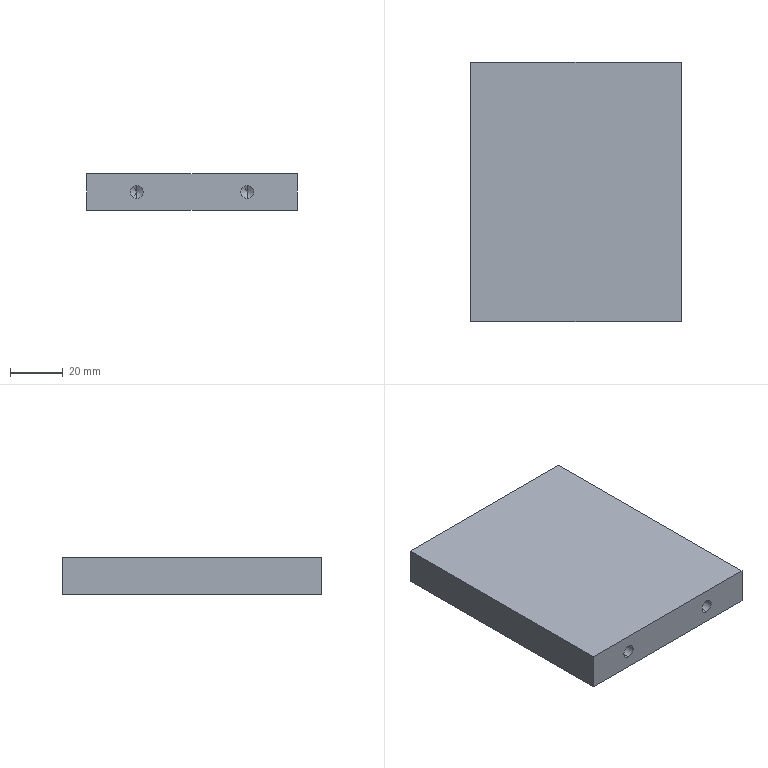Part | SolidWorks | features HoleWzd 2, Extrusion 1 | 1 solid | 22 faces | box 80 x 98.4 x 14 mm | volume 108833 mm3 | cylinder 8 | cone 8 | plane 6 | commonest cylinder face diameters 5 x8
STEP:
#1=CARTESIAN_POINT('',(-17.5,32.2,4.5));
#2=VERTEX_POINT('',#1);
#3=CARTESIAN_POINT('',(-17.5,32.2,9.5));
#4=VERTEX_POINT('',#3);
#5=CARTESIAN_POINT('',(-17.5,32.2,7.));
#6=DIRECTION('',(0.,1.,0.));
#7=DIRECTION('',(0.,0.,1.));
#8=AXIS2_PLACEMENT_3D('',#5,#6,#7);
#9=CIRCLE('',#8,2.5);
#10=EDGE_CURVE('',#2,#4,#9,.T.);
#11=ORIENTED_EDGE('',*,*,#10,.F.);
#12=CARTESIAN_POINT('',(-17.5,49.2,4.5));
#13=VERTEX_POINT('',#12);
#14=CARTESIAN_POINT('',(-17.5,49.2,4.5));
#15=DIRECTION('',(0.,1.,0.));
#16=VECTOR('',#15,1000.);
#17=LINE('',#14,#16);
#18=EDGE_CURVE('',#2,#13,#17,.T.);
#19=ORIENTED_EDGE('',*,*,#18,.T.);
#20=CARTESIAN_POINT('',(-17.5,49.2,9.5));
#21=VERTEX_POINT('',#20);
#22=CARTESIAN_POINT('',(-17.5,49.2,7.));
#23=DIRECTION('',(0.,1.,0.));
#24=DIRECTION('',(0.,0.,1.));
#25=AXIS2_PLACEMENT_3D('',#22,#23,#24);
#26=CIRCLE('',#25,2.5);
#27=EDGE_CURVE('',#13,#21,#26,.T.);
#28=ORIENTED_EDGE('',*,*,#27,.T.);
#29=CARTESIAN_POINT('',(-17.5,49.2,9.5));
#30=DIRECTION('',(0.,1.,0.));
#31=VECTOR('',#30,1000.);
#32=LINE('',#29,#31);
#33=EDGE_CURVE('',#4,#21,#32,.T.);
#34=ORIENTED_EDGE('',*,*,#33,.F.);
#35=EDGE_LOOP('',(#11,#19,#28,#34));
#36=FACE_OUTER_BOUND('',#35,.T.);
#37=CARTESIAN_POINT('',(-17.5,49.2,7.));
#38=DIRECTION('',(0.,1.,0.));
#39=DIRECTION('',(0.,0.,1.));
#40=AXIS2_PLACEMENT_3D('',#37,#38,#39);
#41=CYLINDRICAL_SURFACE('',#40,2.5);
#42=ADVANCED_FACE('',(#36),#41,.F.);
#43=CARTESIAN_POINT('',(-17.5,30.698,7.));
#44=VERTEX_POINT('',#43);
#45=CARTESIAN_POINT('',(-17.5,32.2,9.5));
#46=DIRECTION('',(0.,0.515,0.8572));
#47=VECTOR('',#46,1000.);
#48=LINE('',#45,#47);
#49=EDGE_CURVE('',#44,#4,#48,.T.);
#50=ORIENTED_EDGE('',*,*,#49,.F.);
#51=CARTESIAN_POINT('',(-17.5,32.2,4.5));
#52=DIRECTION('',(0.,0.515,-0.8572));
#53=VECTOR('',#52,1000.);
#54=LINE('',#51,#53);
#55=EDGE_CURVE('',#44,#2,#54,.T.);
#56=ORIENTED_EDGE('',*,*,#55,.T.);
#57=ORIENTED_EDGE('',*,*,#10,.T.);
#58=EDGE_LOOP('',(#50,#56,#57));
#59=FACE_OUTER_BOUND('',#58,.T.);
#60=CARTESIAN_POINT('',(-17.5,32.2,7.));
#61=DIRECTION('',(0.,1.,0.));
#62=DIRECTION('',(0.,0.,1.));
#63=AXIS2_PLACEMENT_3D('',#60,#61,#62);
#64=CONICAL_SURFACE('',#63,2.5,1.03);
#65=ADVANCED_FACE('',(#59),#64,.F.);
#66=CARTESIAN_POINT('',(17.5,32.2,4.5));
#67=VERTEX_POINT('',#66);
#68=CARTESIAN_POINT('',(17.5,32.2,9.5));
#69=VERTEX_POINT('',#68);
#70=CARTESIAN_POINT('',(17.5,32.2,7.));
#71=DIRECTION('',(0.,1.,0.));
#72=DIRECTION('',(0.,0.,1.));
#73=AXIS2_PLACEMENT_3D('',#70,#71,#72);
#74=CIRCLE('',#73,2.5);
#75=EDGE_CURVE('',#67,#69,#74,.T.);
#76=ORIENTED_EDGE('',*,*,#75,.F.);
#77=CARTESIAN_POINT('',(17.5,49.2,4.5));
#78=VERTEX_POINT('',#77);
#79=CARTESIAN_POINT('',(17.5,49.2,4.5));
#80=DIRECTION('',(0.,1.,0.));
#81=VECTOR('',#80,1000.);
#82=LINE('',#79,#81);
#83=EDGE_CURVE('',#67,#78,#82,.T.);
#84=ORIENTED_EDGE('',*,*,#83,.T.);
#85=CARTESIAN_POINT('',(17.5,49.2,9.5));
#86=VERTEX_POINT('',#85);
#87=CARTESIAN_POINT('',(17.5,49.2,7.));
#88=DIRECTION('',(0.,1.,0.));
#89=DIRECTION('',(0.,0.,1.));
#90=AXIS2_PLACEMENT_3D('',#87,#88,#89);
#91=CIRCLE('',#90,2.5);
#92=EDGE_CURVE('',#78,#86,#91,.T.);
#93=ORIENTED_EDGE('',*,*,#92,.T.);
#94=CARTESIAN_POINT('',(17.5,49.2,9.5));
#95=DIRECTION('',(0.,1.,0.));
#96=VECTOR('',#95,1000.);
#97=LINE('',#94,#96);
#98=EDGE_CURVE('',#69,#86,#97,.T.);
#99=ORIENTED_EDGE('',*,*,#98,.F.);
#100=EDGE_LOOP('',(#76,#84,#93,#99));
#101=FACE_OUTER_BOUND('',#100,.T.);
#102=CARTESIAN_POINT('',(17.5,49.2,7.));
#103=DIRECTION('',(0.,1.,0.));
#104=DIRECTION('',(0.,0.,1.));
#105=AXIS2_PLACEMENT_3D('',#102,#103,#104);
#106=CYLINDRICAL_SURFACE('',#105,2.5);
#107=ADVANCED_FACE('',(#101),#106,.F.);
#108=CARTESIAN_POINT('',(17.5,30.698,7.));
#109=VERTEX_POINT('',#108);
#110=CARTESIAN_POINT('',(17.5,32.2,9.5));
#111=DIRECTION('',(0.,0.515,0.8572));
#112=VECTOR('',#111,1000.);
#113=LINE('',#110,#112);
#114=EDGE_CURVE('',#109,#69,#113,.T.);
#115=ORIENTED_EDGE('',*,*,#114,.F.);
#116=CARTESIAN_POINT('',(17.5,32.2,4.5));
#117=DIRECTION('',(0.,0.515,-0.8572));
#118=VECTOR('',#117,1000.);
#119=LINE('',#116,#118);
#120=EDGE_CURVE('',#109,#67,#119,.T.);
#121=ORIENTED_EDGE('',*,*,#120,.T.);
#122=ORIENTED_EDGE('',*,*,#75,.T.);
#123=EDGE_LOOP('',(#115,#121,#122));
#124=FACE_OUTER_BOUND('',#123,.T.);
#125=CARTESIAN_POINT('',(17.5,32.2,7.));
#126=DIRECTION('',(0.,1.,0.));
#127=DIRECTION('',(0.,0.,1.));
#128=AXIS2_PLACEMENT_3D('',#125,#126,#127);
#129=CONICAL_SURFACE('',#128,2.5,1.03);
#130=ADVANCED_FACE('',(#124),#129,.F.);
#131=CARTESIAN_POINT('',(21.,-32.2,9.5));
#132=VERTEX_POINT('',#131);
#133=CARTESIAN_POINT('',(21.,-32.2,4.5));
#134=VERTEX_POINT('',#133);
#135=CARTESIAN_POINT('',(21.,-32.2,7.));
#136=DIRECTION('',(0.,-1.,0.));
#137=DIRECTION('',(0.,0.,-1.));
#138=AXIS2_PLACEMENT_3D('',#135,#136,#137);
#139=CIRCLE('',#138,2.5);
#140=EDGE_CURVE('',#132,#134,#139,.T.);
#141=ORIENTED_EDGE('',*,*,#140,.F.);
#142=CARTESIAN_POINT('',(21.,-49.2,9.5));
#143=VERTEX_POINT('',#142);
#144=CARTESIAN_POINT('',(21.,-49.2,9.5));
#145=DIRECTION('',(0.,-1.,0.));
#146=VECTOR('',#145,1000.);
#147=LINE('',#144,#146);
#148=EDGE_CURVE('',#132,#143,#147,.T.);
#149=ORIENTED_EDGE('',*,*,#148,.T.);
#150=CARTESIAN_POINT('',(21.,-49.2,4.5));
#151=VERTEX_POINT('',#150);
#152=CARTESIAN_POINT('',(21.,-49.2,7.));
#153=DIRECTION('',(0.,-1.,0.));
#154=DIRECTION('',(0.,0.,-1.));
#155=AXIS2_PLACEMENT_3D('',#152,#153,#154);
#156=CIRCLE('',#155,2.5);
#157=EDGE_CURVE('',#143,#151,#156,.T.);
#158=ORIENTED_EDGE('',*,*,#157,.T.);
#159=CARTESIAN_POINT('',(21.,-49.2,4.5));
#160=DIRECTION('',(0.,-1.,0.));
#161=VECTOR('',#160,1000.);
#162=LINE('',#159,#161);
#163=EDGE_CURVE('',#134,#151,#162,.T.);
#164=ORIENTED_EDGE('',*,*,#163,.F.);
#165=EDGE_LOOP('',(#141,#149,#158,#164));
#166=FACE_OUTER_BOUND('',#165,.T.);
#167=CARTESIAN_POINT('',(21.,-49.2,7.));
#168=DIRECTION('',(0.,-1.,0.));
#169=DIRECTION('',(0.,0.,-1.));
#170=AXIS2_PLACEMENT_3D('',#167,#168,#169);
#171=CYLINDRICAL_SURFACE('',#170,2.5);
#172=ADVANCED_FACE('',(#166),#171,.F.);
#173=CARTESIAN_POINT('',(21.,-30.698,7.));
#174=VERTEX_POINT('',#173);
#175=CARTESIAN_POINT('',(21.,-32.2,4.5));
#176=DIRECTION('',(0.,-0.515,-0.8572));
#177=VECTOR('',#176,1000.);
#178=LINE('',#175,#177);
#179=EDGE_CURVE('',#174,#134,#178,.T.);
#180=ORIENTED_EDGE('',*,*,#179,.F.);
#181=CARTESIAN_POINT('',(21.,-32.2,9.5));
#182=DIRECTION('',(0.,-0.515,0.8572));
#183=VECTOR('',#182,1000.);
#184=LINE('',#181,#183);
#185=EDGE_CURVE('',#174,#132,#184,.T.);
#186=ORIENTED_EDGE('',*,*,#185,.T.);
#187=ORIENTED_EDGE('',*,*,#140,.T.);
#188=EDGE_LOOP('',(#180,#186,#187));
#189=FACE_OUTER_BOUND('',#188,.T.);
#190=CARTESIAN_POINT('',(21.,-32.2,7.));
#191=DIRECTION('',(0.,-1.,0.));
#192=DIRECTION('',(0.,0.,-1.));
#193=AXIS2_PLACEMENT_3D('',#190,#191,#192);
#194=CONICAL_SURFACE('',#193,2.5,1.03);
#195=ADVANCED_FACE('',(#189),#194,.F.);
#196=CARTESIAN_POINT('',(-21.,-32.2,9.5));
#197=VERTEX_POINT('',#196);
#198=CARTESIAN_POINT('',(-21.,-32.2,4.5));
#199=VERTEX_POINT('',#198);
#200=CARTESIAN_POINT('',(-21.,-32.2,7.));
#201=DIRECTION('',(0.,-1.,0.));
#202=DIRECTION('',(0.,0.,-1.));
#203=AXIS2_PLACEMENT_3D('',#200,#201,#202);
#204=CIRCLE('',#203,2.5);
#205=EDGE_CURVE('',#197,#199,#204,.T.);
#206=ORIENTED_EDGE('',*,*,#205,.F.);
#207=CARTESIAN_POINT('',(-21.,-49.2,9.5));
#208=VERTEX_POINT('',#207);
#209=CARTESIAN_POINT('',(-21.,-49.2,9.5));
#210=DIRECTION('',(0.,-1.,0.));
#211=VECTOR('',#210,1000.);
#212=LINE('',#209,#211);
#213=EDGE_CURVE('',#197,#208,#212,.T.);
#214=ORIENTED_EDGE('',*,*,#213,.T.);
#215=CARTESIAN_POINT('',(-21.,-49.2,4.5));
#216=VERTEX_POINT('',#215);
#217=CARTESIAN_POINT('',(-21.,-49.2,7.));
#218=DIRECTION('',(0.,-1.,0.));
#219=DIRECTION('',(0.,0.,-1.));
#220=AXIS2_PLACEMENT_3D('',#217,#218,#219);
#221=CIRCLE('',#220,2.5);
#222=EDGE_CURVE('',#208,#216,#221,.T.);
#223=ORIENTED_EDGE('',*,*,#222,.T.);
#224=CARTESIAN_POINT('',(-21.,-49.2,4.5));
#225=DIRECTION('',(0.,-1.,0.));
#226=VECTOR('',#225,1000.);
#227=LINE('',#224,#226);
#228=EDGE_CURVE('',#199,#216,#227,.T.);
#229=ORIENTED_EDGE('',*,*,#228,.F.);
#230=EDGE_LOOP('',(#206,#214,#223,#229));
#231=FACE_OUTER_BOUND('',#230,.T.);
#232=CARTESIAN_POINT('',(-21.,-49.2,7.));
#233=DIRECTION('',(0.,-1.,0.));
#234=DIRECTION('',(0.,0.,-1.));
#235=AXIS2_PLACEMENT_3D('',#232,#233,#234);
#236=CYLINDRICAL_SURFACE('',#235,2.5);
#237=ADVANCED_FACE('',(#231),#236,.F.);
#238=CARTESIAN_POINT('',(-21.,-30.698,7.));
#239=VERTEX_POINT('',#238);
#240=CARTESIAN_POINT('',(-21.,-32.2,4.5));
#241=DIRECTION('',(0.,-0.515,-0.8572));
#242=VECTOR('',#241,1000.);
#243=LINE('',#240,#242);
#244=EDGE_CURVE('',#239,#199,#243,.T.);
#245=ORIENTED_EDGE('',*,*,#244,.F.);
#246=CARTESIAN_POINT('',(-21.,-32.2,9.5));
#247=DIRECTION('',(0.,-0.515,0.8572));
#248=VECTOR('',#247,1000.);
#249=LINE('',#246,#248);
#250=EDGE_CURVE('',#239,#197,#249,.T.);
#251=ORIENTED_EDGE('',*,*,#250,.T.);
#252=ORIENTED_EDGE('',*,*,#205,.T.);
#253=EDGE_LOOP('',(#245,#251,#252));
#254=FACE_OUTER_BOUND('',#253,.T.);
#255=CARTESIAN_POINT('',(-21.,-32.2,7.));
#256=DIRECTION('',(0.,-1.,0.));
#257=DIRECTION('',(0.,0.,-1.));
#258=AXIS2_PLACEMENT_3D('',#255,#256,#257);
#259=CONICAL_SURFACE('',#258,2.5,1.03);
#260=ADVANCED_FACE('',(#254),#259,.F.);
#261=CARTESIAN_POINT('',(40.,-49.2,0.));
#262=VERTEX_POINT('',#261);
#263=CARTESIAN_POINT('',(40.,49.2,0.));
#264=VERTEX_POINT('',#263);
#265=CARTESIAN_POINT('',(40.,49.2,0.));
#266=DIRECTION('',(0.,1.,0.));
#267=VECTOR('',#266,1000.);
#268=LINE('',#265,#267);
#269=EDGE_CURVE('',#262,#264,#268,.T.);
#270=ORIENTED_EDGE('',*,*,#269,.T.);
#271=CARTESIAN_POINT('',(40.,49.2,14.));
#272=VERTEX_POINT('',#271);
#273=CARTESIAN_POINT('',(40.,49.2,14.));
#274=DIRECTION('',(0.,0.,-1.));
#275=VECTOR('',#274,1000.);
#276=LINE('',#273,#275);
#277=EDGE_CURVE('',#272,#264,#276,.T.);
#278=ORIENTED_EDGE('',*,*,#277,.F.);
#279=CARTESIAN_POINT('',(40.,-49.2,14.));
#280=VERTEX_POINT('',#279);
#281=CARTESIAN_POINT('',(40.,49.2,14.));
#282=DIRECTION('',(0.,1.,0.));
#283=VECTOR('',#282,1000.);
#284=LINE('',#281,#283);
#285=EDGE_CURVE('',#280,#272,#284,.T.);
#286=ORIENTED_EDGE('',*,*,#285,.F.);
#287=CARTESIAN_POINT('',(40.,-49.2,14.));
#288=DIRECTION('',(0.,0.,-1.));
#289=VECTOR('',#288,1000.);
#290=LINE('',#287,#289);
#291=EDGE_CURVE('',#280,#262,#290,.T.);
#292=ORIENTED_EDGE('',*,*,#291,.T.);
#293=EDGE_LOOP('',(#270,#278,#286,#292));
#294=FACE_OUTER_BOUND('',#293,.T.);
#295=CARTESIAN_POINT('',(40.,49.2,14.));
#296=DIRECTION('',(-1.,0.,0.));
#297=DIRECTION('',(0.,-1.,0.));
#298=AXIS2_PLACEMENT_3D('',#295,#296,#297);
#299=PLANE('',#298);
#300=ADVANCED_FACE('',(#294),#299,.F.);
#301=CARTESIAN_POINT('',(-17.5,49.2,7.));
#302=DIRECTION('',(0.,1.,0.));
#303=DIRECTION('',(0.,0.,1.));
#304=AXIS2_PLACEMENT_3D('',#301,#302,#303);
#305=CIRCLE('',#304,2.5);
#306=EDGE_CURVE('',#21,#13,#305,.T.);
#307=ORIENTED_EDGE('',*,*,#306,.F.);
#308=ORIENTED_EDGE('',*,*,#27,.F.);
#309=EDGE_LOOP('',(#307,#308));
#310=FACE_BOUND('',#309,.T.);
#311=CARTESIAN_POINT('',(17.5,49.2,7.));
#312=DIRECTION('',(0.,1.,0.));
#313=DIRECTION('',(0.,0.,1.));
#314=AXIS2_PLACEMENT_3D('',#311,#312,#313);
#315=CIRCLE('',#314,2.5);
#316=EDGE_CURVE('',#86,#78,#315,.T.);
#317=ORIENTED_EDGE('',*,*,#316,.F.);
#318=ORIENTED_EDGE('',*,*,#92,.F.);
#319=EDGE_LOOP('',(#317,#318));
#320=FACE_BOUND('',#319,.T.);
#321=CARTESIAN_POINT('',(-40.,49.2,0.));
#322=VERTEX_POINT('',#321);
#323=CARTESIAN_POINT('',(-40.,49.2,0.));
#324=DIRECTION('',(-1.,0.,0.));
#325=VECTOR('',#324,1000.);
#326=LINE('',#323,#325);
#327=EDGE_CURVE('',#264,#322,#326,.T.);
#328=ORIENTED_EDGE('',*,*,#327,.T.);
#329=CARTESIAN_POINT('',(-40.,49.2,14.));
#330=VERTEX_POINT('',#329);
#331=CARTESIAN_POINT('',(-40.,49.2,14.));
#332=DIRECTION('',(0.,0.,-1.));
#333=VECTOR('',#332,1000.);
#334=LINE('',#331,#333);
#335=EDGE_CURVE('',#330,#322,#334,.T.);
#336=ORIENTED_EDGE('',*,*,#335,.F.);
#337=CARTESIAN_POINT('',(-40.,49.2,14.));
#338=DIRECTION('',(-1.,0.,0.));
#339=VECTOR('',#338,1000.);
#340=LINE('',#337,#339);
#341=EDGE_CURVE('',#272,#330,#340,.T.);
#342=ORIENTED_EDGE('',*,*,#341,.F.);
#343=ORIENTED_EDGE('',*,*,#277,.T.);
#344=EDGE_LOOP('',(#328,#336,#342,#343));
#345=FACE_OUTER_BOUND('',#344,.T.);
#346=CARTESIAN_POINT('',(-40.,49.2,14.));
#347=DIRECTION('',(0.,-1.,0.));
#348=DIRECTION('',(0.,0.,-1.));
#349=AXIS2_PLACEMENT_3D('',#346,#347,#348);
#350=PLANE('',#349);
#351=ADVANCED_FACE('',(#310,#320,#345),#350,.F.);
#352=CARTESIAN_POINT('',(-40.,-49.2,0.));
#353=VERTEX_POINT('',#352);
#354=CARTESIAN_POINT('',(-40.,49.2,0.));
#355=DIRECTION('',(0.,-1.,0.));
#356=VECTOR('',#355,1000.);
#357=LINE('',#354,#356);
#358=EDGE_CURVE('',#322,#353,#357,.T.);
#359=ORIENTED_EDGE('',*,*,#358,.T.);
#360=CARTESIAN_POINT('',(-40.,-49.2,14.));
#361=VERTEX_POINT('',#360);
#362=CARTESIAN_POINT('',(-40.,-49.2,14.));
#363=DIRECTION('',(0.,0.,-1.));
#364=VECTOR('',#363,1000.);
#365=LINE('',#362,#364);
#366=EDGE_CURVE('',#361,#353,#365,.T.);
#367=ORIENTED_EDGE('',*,*,#366,.F.);
#368=CARTESIAN_POINT('',(-40.,49.2,14.));
#369=DIRECTION('',(0.,-1.,0.));
#370=VECTOR('',#369,1000.);
#371=LINE('',#368,#370);
#372=EDGE_CURVE('',#330,#361,#371,.T.);
#373=ORIENTED_EDGE('',*,*,#372,.F.);
#374=ORIENTED_EDGE('',*,*,#335,.T.);
#375=EDGE_LOOP('',(#359,#367,#373,#374));
#376=FACE_OUTER_BOUND('',#375,.T.);
#377=CARTESIAN_POINT('',(-40.,49.2,14.));
#378=DIRECTION('',(1.,0.,0.));
#379=DIRECTION('',(0.,1.,0.));
#380=AXIS2_PLACEMENT_3D('',#377,#378,#379);
#381=PLANE('',#380);
#382=ADVANCED_FACE('',(#376),#381,.F.);
#383=CARTESIAN_POINT('',(21.,-49.2,7.));
#384=DIRECTION('',(0.,-1.,0.));
#385=DIRECTION('',(0.,0.,-1.));
#386=AXIS2_PLACEMENT_3D('',#383,#384,#385);
#387=CIRCLE('',#386,2.5);
#388=EDGE_CURVE('',#151,#143,#387,.T.);
#389=ORIENTED_EDGE('',*,*,#388,.F.);
#390=ORIENTED_EDGE('',*,*,#157,.F.);
#391=EDGE_LOOP('',(#389,#390));
#392=FACE_BOUND('',#391,.T.);
#393=CARTESIAN_POINT('',(-21.,-49.2,7.));
#394=DIRECTION('',(0.,-1.,0.));
#395=DIRECTION('',(0.,0.,-1.));
#396=AXIS2_PLACEMENT_3D('',#393,#394,#395);
#397=CIRCLE('',#396,2.5);
#398=EDGE_CURVE('',#216,#208,#397,.T.);
#399=ORIENTED_EDGE('',*,*,#398,.F.);
#400=ORIENTED_EDGE('',*,*,#222,.F.);
#401=EDGE_LOOP('',(#399,#400));
#402=FACE_BOUND('',#401,.T.);
#403=CARTESIAN_POINT('',(-40.,-49.2,0.));
#404=DIRECTION('',(1.,0.,0.));
#405=VECTOR('',#404,1000.);
#406=LINE('',#403,#405);
#407=EDGE_CURVE('',#353,#262,#406,.T.);
#408=ORIENTED_EDGE('',*,*,#407,.T.);
#409=ORIENTED_EDGE('',*,*,#291,.F.);
#410=CARTESIAN_POINT('',(-40.,-49.2,14.));
#411=DIRECTION('',(1.,0.,0.));
#412=VECTOR('',#411,1000.);
#413=LINE('',#410,#412);
#414=EDGE_CURVE('',#361,#280,#413,.T.);
#415=ORIENTED_EDGE('',*,*,#414,.F.);
#416=ORIENTED_EDGE('',*,*,#366,.T.);
#417=EDGE_LOOP('',(#408,#409,#415,#416));
#418=FACE_OUTER_BOUND('',#417,.T.);
#419=CARTESIAN_POINT('',(-40.,-49.2,14.));
#420=DIRECTION('',(0.,1.,0.));
#421=DIRECTION('',(0.,0.,1.));
#422=AXIS2_PLACEMENT_3D('',#419,#420,#421);
#423=PLANE('',#422);
#424=ADVANCED_FACE('',(#392,#402,#418),#423,.F.);
#425=ORIENTED_EDGE('',*,*,#285,.T.);
#426=ORIENTED_EDGE('',*,*,#341,.T.);
#427=ORIENTED_EDGE('',*,*,#372,.T.);
#428=ORIENTED_EDGE('',*,*,#414,.T.);
#429=EDGE_LOOP('',(#425,#426,#427,#428));
#430=FACE_OUTER_BOUND('',#429,.T.);
#431=CARTESIAN_POINT('',(0.,0.,14.));
#432=DIRECTION('',(0.,0.,1.));
#433=DIRECTION('',(1.,0.,0.));
#434=AXIS2_PLACEMENT_3D('',#431,#432,#433);
#435=PLANE('',#434);
#436=ADVANCED_FACE('',(#430),#435,.T.);
#437=ORIENTED_EDGE('',*,*,#269,.F.);
#438=ORIENTED_EDGE('',*,*,#407,.F.);
#439=ORIENTED_EDGE('',*,*,#358,.F.);
#440=ORIENTED_EDGE('',*,*,#327,.F.);
#441=EDGE_LOOP('',(#437,#438,#439,#440));
#442=FACE_OUTER_BOUND('',#441,.T.);
#443=CARTESIAN_POINT('',(0.,0.,0.));
#444=DIRECTION('',(0.,0.,1.));
#445=DIRECTION('',(1.,0.,0.));
#446=AXIS2_PLACEMENT_3D('',#443,#444,#445);
#447=PLANE('',#446);
#448=ADVANCED_FACE('',(#442),#447,.F.);
#449=ORIENTED_EDGE('',*,*,#250,.F.);
#450=ORIENTED_EDGE('',*,*,#244,.T.);
#451=CARTESIAN_POINT('',(-21.,-32.2,7.));
#452=DIRECTION('',(0.,-1.,0.));
#453=DIRECTION('',(0.,0.,-1.));
#454=AXIS2_PLACEMENT_3D('',#451,#452,#453);
#455=CIRCLE('',#454,2.5);
#456=EDGE_CURVE('',#199,#197,#455,.T.);
#457=ORIENTED_EDGE('',*,*,#456,.T.);
#458=EDGE_LOOP('',(#449,#450,#457));
#459=FACE_OUTER_BOUND('',#458,.T.);
#460=CARTESIAN_POINT('',(-21.,-32.2,7.));
#461=DIRECTION('',(0.,-1.,0.));
#462=DIRECTION('',(0.,0.,-1.));
#463=AXIS2_PLACEMENT_3D('',#460,#461,#462);
#464=CONICAL_SURFACE('',#463,2.5,1.03);
#465=ADVANCED_FACE('',(#459),#464,.F.);
#466=ORIENTED_EDGE('',*,*,#213,.F.);
#467=ORIENTED_EDGE('',*,*,#456,.F.);
#468=ORIENTED_EDGE('',*,*,#228,.T.);
#469=ORIENTED_EDGE('',*,*,#398,.T.);
#470=EDGE_LOOP('',(#466,#467,#468,#469));
#471=FACE_OUTER_BOUND('',#470,.T.);
#472=CARTESIAN_POINT('',(-21.,-49.2,7.));
#473=DIRECTION('',(0.,-1.,0.));
#474=DIRECTION('',(0.,0.,-1.));
#475=AXIS2_PLACEMENT_3D('',#472,#473,#474);
#476=CYLINDRICAL_SURFACE('',#475,2.5);
#477=ADVANCED_FACE('',(#471),#476,.F.);
#478=ORIENTED_EDGE('',*,*,#185,.F.);
#479=ORIENTED_EDGE('',*,*,#179,.T.);
#480=CARTESIAN_POINT('',(21.,-32.2,7.));
#481=DIRECTION('',(0.,-1.,0.));
#482=DIRECTION('',(0.,0.,-1.));
#483=AXIS2_PLACEMENT_3D('',#480,#481,#482);
#484=CIRCLE('',#483,2.5);
#485=EDGE_CURVE('',#134,#132,#484,.T.);
#486=ORIENTED_EDGE('',*,*,#485,.T.);
#487=EDGE_LOOP('',(#478,#479,#486));
#488=FACE_OUTER_BOUND('',#487,.T.);
#489=CARTESIAN_POINT('',(21.,-32.2,7.));
#490=DIRECTION('',(0.,-1.,0.));
#491=DIRECTION('',(0.,0.,-1.));
#492=AXIS2_PLACEMENT_3D('',#489,#490,#491);
#493=CONICAL_SURFACE('',#492,2.5,1.03);
#494=ADVANCED_FACE('',(#488),#493,.F.);
#495=ORIENTED_EDGE('',*,*,#148,.F.);
#496=ORIENTED_EDGE('',*,*,#485,.F.);
#497=ORIENTED_EDGE('',*,*,#163,.T.);
#498=ORIENTED_EDGE('',*,*,#388,.T.);
#499=EDGE_LOOP('',(#495,#496,#497,#498));
#500=FACE_OUTER_BOUND('',#499,.T.);
#501=CARTESIAN_POINT('',(21.,-49.2,7.));
#502=DIRECTION('',(0.,-1.,0.));
#503=DIRECTION('',(0.,0.,-1.));
#504=AXIS2_PLACEMENT_3D('',#501,#502,#503);
#505=CYLINDRICAL_SURFACE('',#504,2.5);
#506=ADVANCED_FACE('',(#500),#505,.F.);
#507=ORIENTED_EDGE('',*,*,#120,.F.);
#508=ORIENTED_EDGE('',*,*,#114,.T.);
#509=CARTESIAN_POINT('',(17.5,32.2,7.));
#510=DIRECTION('',(0.,1.,0.));
#511=DIRECTION('',(0.,0.,1.));
#512=AXIS2_PLACEMENT_3D('',#509,#510,#511);
#513=CIRCLE('',#512,2.5);
#514=EDGE_CURVE('',#69,#67,#513,.T.);
#515=ORIENTED_EDGE('',*,*,#514,.T.);
#516=EDGE_LOOP('',(#507,#508,#515));
#517=FACE_OUTER_BOUND('',#516,.T.);
#518=CARTESIAN_POINT('',(17.5,32.2,7.));
#519=DIRECTION('',(0.,1.,0.));
#520=DIRECTION('',(0.,0.,1.));
#521=AXIS2_PLACEMENT_3D('',#518,#519,#520);
#522=CONICAL_SURFACE('',#521,2.5,1.03);
#523=ADVANCED_FACE('',(#517),#522,.F.);
#524=ORIENTED_EDGE('',*,*,#83,.F.);
#525=ORIENTED_EDGE('',*,*,#514,.F.);
#526=ORIENTED_EDGE('',*,*,#98,.T.);
#527=ORIENTED_EDGE('',*,*,#316,.T.);
#528=EDGE_LOOP('',(#524,#525,#526,#527));
#529=FACE_OUTER_BOUND('',#528,.T.);
#530=CARTESIAN_POINT('',(17.5,49.2,7.));
#531=DIRECTION('',(0.,1.,0.));
#532=DIRECTION('',(0.,0.,1.));
#533=AXIS2_PLACEMENT_3D('',#530,#531,#532);
#534=CYLINDRICAL_SURFACE('',#533,2.5);
#535=ADVANCED_FACE('',(#529),#534,.F.);
#536=ORIENTED_EDGE('',*,*,#55,.F.);
#537=ORIENTED_EDGE('',*,*,#49,.T.);
#538=CARTESIAN_POINT('',(-17.5,32.2,7.));
#539=DIRECTION('',(0.,1.,0.));
#540=DIRECTION('',(0.,0.,1.));
#541=AXIS2_PLACEMENT_3D('',#538,#539,#540);
#542=CIRCLE('',#541,2.5);
#543=EDGE_CURVE('',#4,#2,#542,.T.);
#544=ORIENTED_EDGE('',*,*,#543,.T.);
#545=EDGE_LOOP('',(#536,#537,#544));
#546=FACE_OUTER_BOUND('',#545,.T.);
#547=CARTESIAN_POINT('',(-17.5,32.2,7.));
#548=DIRECTION('',(0.,1.,0.));
#549=DIRECTION('',(0.,0.,1.));
#550=AXIS2_PLACEMENT_3D('',#547,#548,#549);
#551=CONICAL_SURFACE('',#550,2.5,1.03);
#552=ADVANCED_FACE('',(#546),#551,.F.);
#553=ORIENTED_EDGE('',*,*,#18,.F.);
#554=ORIENTED_EDGE('',*,*,#543,.F.);
#555=ORIENTED_EDGE('',*,*,#33,.T.);
#556=ORIENTED_EDGE('',*,*,#306,.T.);
#557=EDGE_LOOP('',(#553,#554,#555,#556));
#558=FACE_OUTER_BOUND('',#557,.T.);
#559=CARTESIAN_POINT('',(-17.5,49.2,7.));
#560=DIRECTION('',(0.,1.,0.));
#561=DIRECTION('',(0.,0.,1.));
#562=AXIS2_PLACEMENT_3D('',#559,#560,#561);
#563=CYLINDRICAL_SURFACE('',#562,2.5);
#564=ADVANCED_FACE('',(#558),#563,.F.);
#565=CLOSED_SHELL('',(#42,#65,#107,#130,#172,#195,#237,#260,#300,#351,#382,#424,#436,#448,#465,#477,#494,#506,#523,#535,#552,#564));
#566=MANIFOLD_SOLID_BREP('',#565);
#567=CARTESIAN_POINT('',(0.,0.,0.));
#568=DIRECTION('',(0.,0.,1.));
#569=DIRECTION('',(1.,0.,0.));
#570=AXIS2_PLACEMENT_3D('',#567,#568,#569);
#571=(LENGTH_UNIT()NAMED_UNIT(*)SI_UNIT(.MILLI.,.METRE.));
#572=UNCERTAINTY_MEASURE_WITH_UNIT(LENGTH_MEASURE(0.00001),#571,'','');
#573=(NAMED_UNIT(*)PLANE_ANGLE_UNIT()SI_UNIT($,.RADIAN.));
#574=(NAMED_UNIT(*)SI_UNIT($,.STERADIAN.)SOLID_ANGLE_UNIT());
#575=(GEOMETRIC_REPRESENTATION_CONTEXT(3)GLOBAL_UNCERTAINTY_ASSIGNED_CONTEXT((#572))GLOBAL_UNIT_ASSIGNED_CONTEXT((#571,#573,#574))REPRESENTATION_CONTEXT('',''));
#576=ADVANCED_BREP_SHAPE_REPRESENTATION('',(#566,#570),#575);